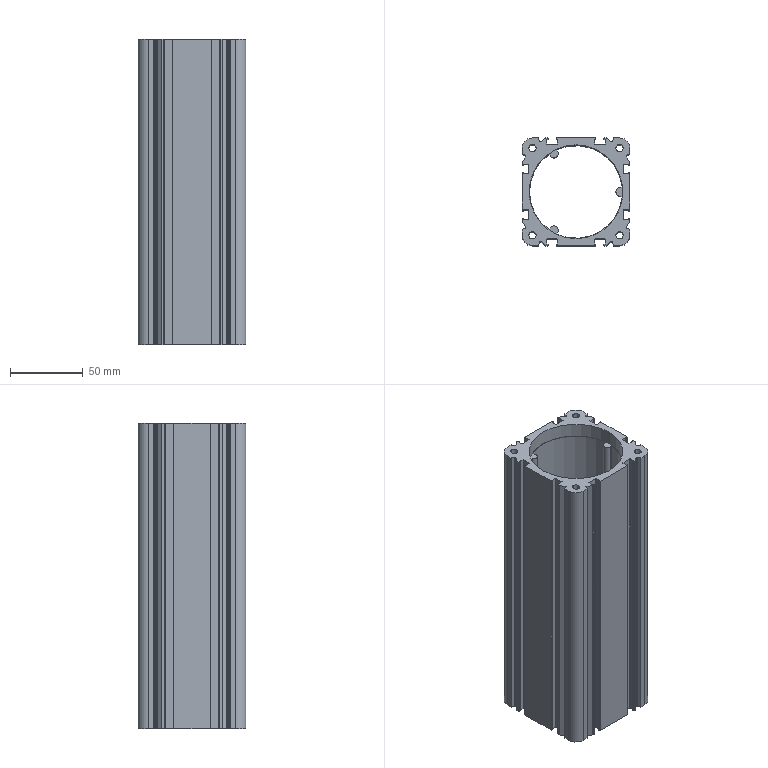Part | SolidWorks | features BaseBody 1 | 1 solid | 190 faces | box 74 x 74 x 210 mm | volume 398957 mm3 | plane 110 | cylinder 80 | commonest cylinder face diameters 0.6 x56 5 x8 6 x4 14 x4 64 x4 64.5 x4